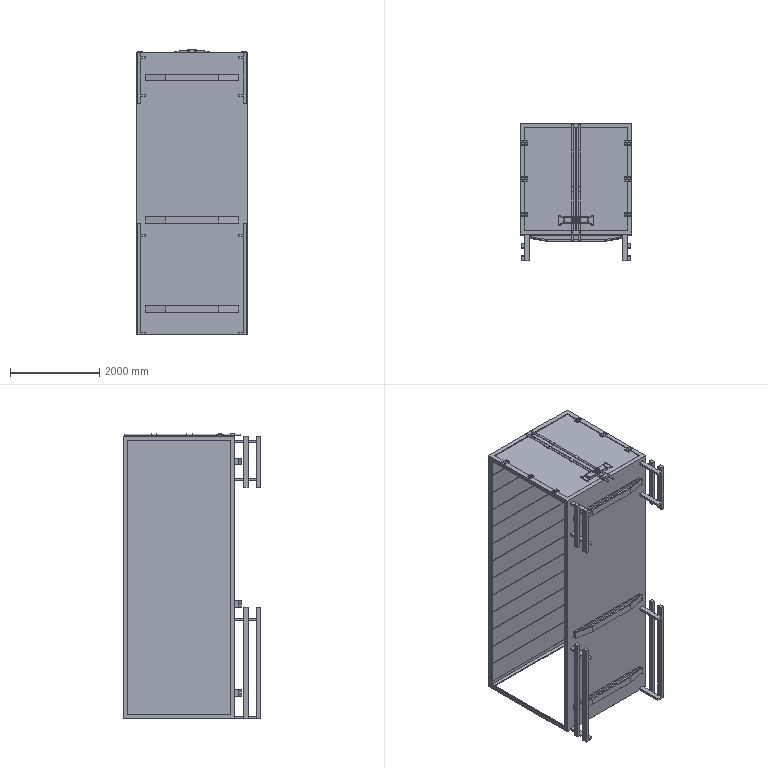Part | STEP file | contener 2_Varsayılan | 3 solids | 1088 faces | box 2500 x 3080 x 6400 mm | volume 75178942 mm3 | plane 856 | cylinder 192 | spline 40 | commonest cylinder face diameters 18 x56 20 x56 23 x24 25 x24 60 x14 40 x12